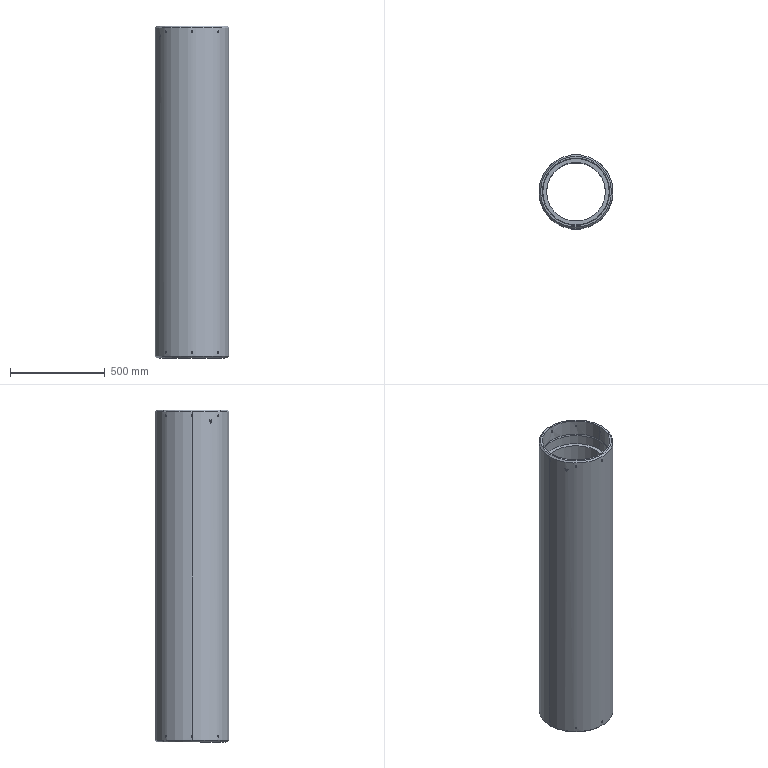Part | NX | features BREP 1 | 1 solid | 76 faces | box 390 x 390 x 1750 mm | volume 70457187 mm3 | cylinder 46 | plane 20 | cone 10 | commonest cylinder face diameters 10.2 x32 350 x4 354.5 x4 390 x4 310 x2